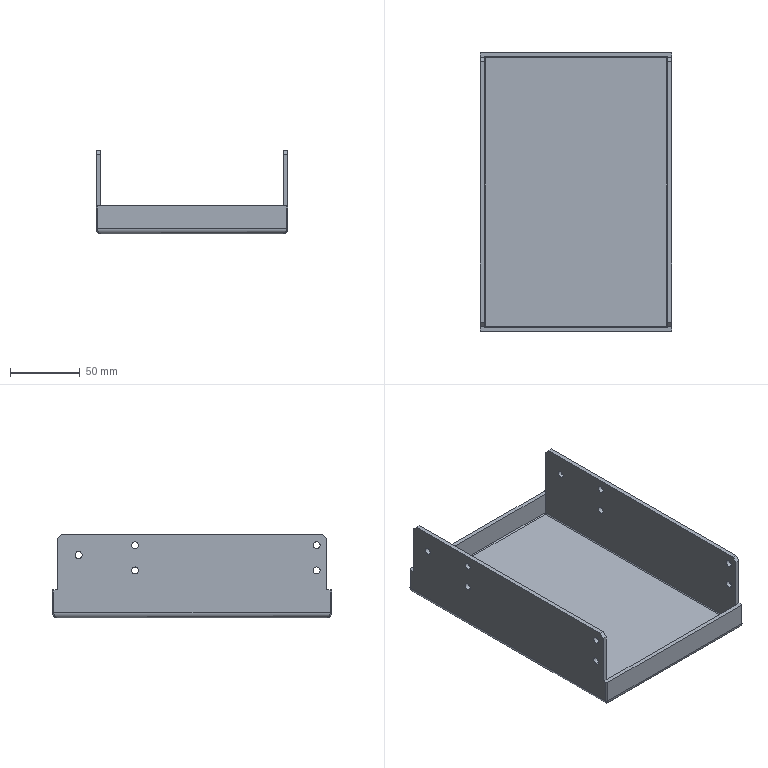Part | STEP file | Seal box | 1 solid | 58 faces | box 137.473 x 200 x 60 mm | volume 159920 mm3 | cylinder 32 | plane 22 | spline 4 | commonest cylinder face diameters 5 x20 1.473 x4 2 x4 7.473 x4